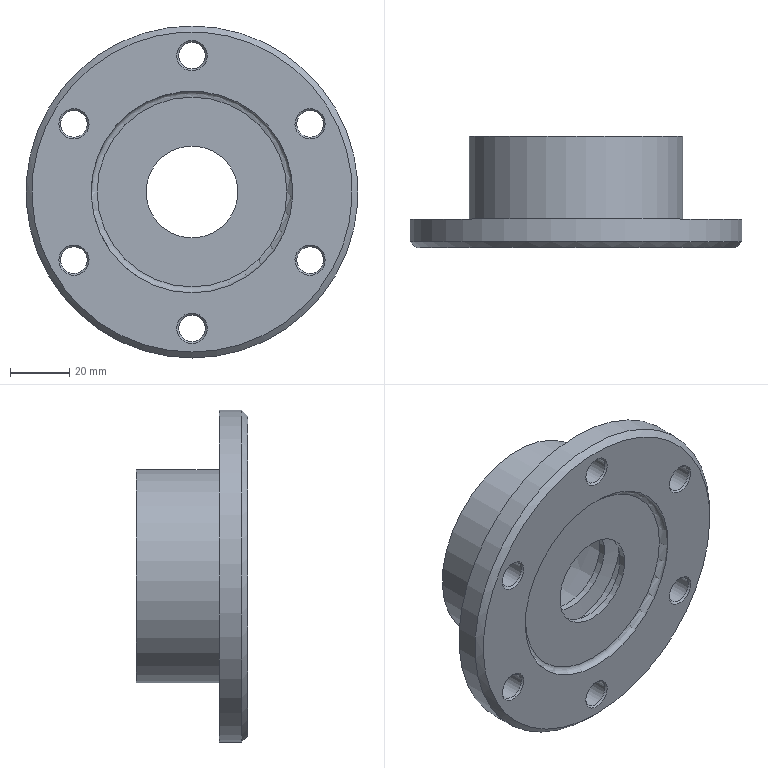Part | NX | 1 solid | 34 faces | box 112 x 37.6 x 112 mm | volume 108254 mm3 | cone 16 | cylinder 11 | plane 5 | torus 2 | commonest cylinder face diameters 9 x6 31 x2 44 x1 72 x1 112 x1
STEP:
#1=CARTESIAN_POINT('',(43.734,-42.624,25.25));
#2=VERTEX_POINT('',#1);
#3=CARTESIAN_POINT('',(39.837,-42.624,23.));
#4=DIRECTION('',(0.,-1.,0.));
#5=DIRECTION('',(0.866,0.,0.5));
#6=AXIS2_PLACEMENT_3D('',#3,#4,#5);
#7=CIRCLE('',#6,4.5);
#8=EDGE_CURVE('',#2,#2,#7,.T.);
#9=ORIENTED_EDGE('',*,*,#8,.F.);
#10=EDGE_LOOP('',(#9));
#11=FACE_BOUND('',#10,.T.);
#12=CARTESIAN_POINT('',(44.254,-43.224,25.55));
#13=VERTEX_POINT('',#12);
#14=CARTESIAN_POINT('',(39.837,-43.224,23.));
#15=DIRECTION('',(0.,1.,0.));
#16=DIRECTION('',(0.866,0.,0.5));
#17=AXIS2_PLACEMENT_3D('',#14,#15,#16);
#18=CIRCLE('',#17,5.1);
#19=EDGE_CURVE('',#13,#13,#18,.T.);
#20=ORIENTED_EDGE('',*,*,#19,.F.);
#21=EDGE_LOOP('',(#20));
#22=FACE_BOUND('',#21,.T.);
#23=CARTESIAN_POINT('',(39.837,-43.224,23.));
#24=DIRECTION('',(0.,-1.,0.));
#25=DIRECTION('',(0.866,0.,0.5));
#26=AXIS2_PLACEMENT_3D('',#23,#24,#25);
#27=CONICAL_SURFACE('',#26,5.1,45.);
#28=ADVANCED_FACE('',(#11,#22),#27,.F.);
#29=CARTESIAN_POINT('',(35.94,-34.224,20.75));
#30=VERTEX_POINT('',#29);
#31=CARTESIAN_POINT('',(39.837,-34.224,23.));
#32=DIRECTION('',(0.,1.,0.));
#33=DIRECTION('',(-0.866,0.,-0.5));
#34=AXIS2_PLACEMENT_3D('',#31,#32,#33);
#35=CIRCLE('',#34,4.5);
#36=EDGE_CURVE('',#30,#30,#35,.T.);
#37=ORIENTED_EDGE('',*,*,#36,.F.);
#38=EDGE_LOOP('',(#37));
#39=FACE_BOUND('',#38,.T.);
#40=CARTESIAN_POINT('',(35.42,-33.624,20.45));
#41=VERTEX_POINT('',#40);
#42=CARTESIAN_POINT('',(39.837,-33.624,23.));
#43=DIRECTION('',(0.,-1.,0.));
#44=DIRECTION('',(-0.866,0.,-0.5));
#45=AXIS2_PLACEMENT_3D('',#42,#43,#44);
#46=CIRCLE('',#45,5.1);
#47=EDGE_CURVE('',#41,#41,#46,.T.);
#48=ORIENTED_EDGE('',*,*,#47,.F.);
#49=EDGE_LOOP('',(#48));
#50=FACE_BOUND('',#49,.T.);
#51=CARTESIAN_POINT('',(39.837,-33.624,23.));
#52=DIRECTION('',(0.,1.,0.));
#53=DIRECTION('',(-0.866,0.,-0.5));
#54=AXIS2_PLACEMENT_3D('',#51,#52,#53);
#55=CONICAL_SURFACE('',#54,5.1,45.);
#56=ADVANCED_FACE('',(#39,#50),#55,.F.);
#57=ORIENTED_EDGE('',*,*,#36,.T.);
#58=EDGE_LOOP('',(#57));
#59=FACE_BOUND('',#58,.T.);
#60=ORIENTED_EDGE('',*,*,#8,.T.);
#61=EDGE_LOOP('',(#60));
#62=FACE_BOUND('',#61,.T.);
#63=CARTESIAN_POINT('',(39.837,-43.224,23.));
#64=DIRECTION('',(0.,1.,0.));
#65=DIRECTION('',(-0.866,0.,-0.5));
#66=AXIS2_PLACEMENT_3D('',#63,#64,#65);
#67=CYLINDRICAL_SURFACE('',#66,4.5);
#68=ADVANCED_FACE('',(#59,#62),#67,.F.);
#69=CARTESIAN_POINT('',(43.734,-42.624,-25.25));
#70=VERTEX_POINT('',#69);
#71=CARTESIAN_POINT('',(39.837,-42.624,-23.));
#72=DIRECTION('',(0.,-1.,0.));
#73=DIRECTION('',(0.866,0.,-0.5));
#74=AXIS2_PLACEMENT_3D('',#71,#72,#73);
#75=CIRCLE('',#74,4.5);
#76=EDGE_CURVE('',#70,#70,#75,.T.);
#77=ORIENTED_EDGE('',*,*,#76,.F.);
#78=EDGE_LOOP('',(#77));
#79=FACE_BOUND('',#78,.T.);
#80=CARTESIAN_POINT('',(44.254,-43.224,-25.55));
#81=VERTEX_POINT('',#80);
#82=CARTESIAN_POINT('',(39.837,-43.224,-23.));
#83=DIRECTION('',(0.,1.,0.));
#84=DIRECTION('',(0.866,0.,-0.5));
#85=AXIS2_PLACEMENT_3D('',#82,#83,#84);
#86=CIRCLE('',#85,5.1);
#87=EDGE_CURVE('',#81,#81,#86,.T.);
#88=ORIENTED_EDGE('',*,*,#87,.F.);
#89=EDGE_LOOP('',(#88));
#90=FACE_BOUND('',#89,.T.);
#91=CARTESIAN_POINT('',(39.837,-43.224,-23.));
#92=DIRECTION('',(0.,-1.,0.));
#93=DIRECTION('',(0.866,0.,-0.5));
#94=AXIS2_PLACEMENT_3D('',#91,#92,#93);
#95=CONICAL_SURFACE('',#94,5.1,45.);
#96=ADVANCED_FACE('',(#79,#90),#95,.F.);
#97=CARTESIAN_POINT('',(35.94,-34.224,-20.75));
#98=VERTEX_POINT('',#97);
#99=CARTESIAN_POINT('',(39.837,-34.224,-23.));
#100=DIRECTION('',(0.,1.,0.));
#101=DIRECTION('',(-0.866,0.,0.5));
#102=AXIS2_PLACEMENT_3D('',#99,#100,#101);
#103=CIRCLE('',#102,4.5);
#104=EDGE_CURVE('',#98,#98,#103,.T.);
#105=ORIENTED_EDGE('',*,*,#104,.F.);
#106=EDGE_LOOP('',(#105));
#107=FACE_BOUND('',#106,.T.);
#108=CARTESIAN_POINT('',(35.42,-33.624,-20.45));
#109=VERTEX_POINT('',#108);
#110=CARTESIAN_POINT('',(39.837,-33.624,-23.));
#111=DIRECTION('',(0.,-1.,0.));
#112=DIRECTION('',(-0.866,0.,0.5));
#113=AXIS2_PLACEMENT_3D('',#110,#111,#112);
#114=CIRCLE('',#113,5.1);
#115=EDGE_CURVE('',#109,#109,#114,.T.);
#116=ORIENTED_EDGE('',*,*,#115,.F.);
#117=EDGE_LOOP('',(#116));
#118=FACE_BOUND('',#117,.T.);
#119=CARTESIAN_POINT('',(39.837,-33.624,-23.));
#120=DIRECTION('',(0.,1.,0.));
#121=DIRECTION('',(-0.866,0.,0.5));
#122=AXIS2_PLACEMENT_3D('',#119,#120,#121);
#123=CONICAL_SURFACE('',#122,5.1,45.);
#124=ADVANCED_FACE('',(#107,#118),#123,.F.);
#125=ORIENTED_EDGE('',*,*,#104,.T.);
#126=EDGE_LOOP('',(#125));
#127=FACE_BOUND('',#126,.T.);
#128=ORIENTED_EDGE('',*,*,#76,.T.);
#129=EDGE_LOOP('',(#128));
#130=FACE_BOUND('',#129,.T.);
#131=CARTESIAN_POINT('',(39.837,-43.224,-23.));
#132=DIRECTION('',(0.,1.,0.));
#133=DIRECTION('',(-0.866,0.,0.5));
#134=AXIS2_PLACEMENT_3D('',#131,#132,#133);
#135=CYLINDRICAL_SURFACE('',#134,4.5);
#136=ADVANCED_FACE('',(#127,#130),#135,.F.);
#137=CARTESIAN_POINT('',(0.,-42.624,-50.5));
#138=VERTEX_POINT('',#137);
#139=CARTESIAN_POINT('',(0.,-42.624,-46.));
#140=DIRECTION('',(0.,-1.,0.));
#141=DIRECTION('',(0.,0.,-1.));
#142=AXIS2_PLACEMENT_3D('',#139,#140,#141);
#143=CIRCLE('',#142,4.5);
#144=EDGE_CURVE('',#138,#138,#143,.T.);
#145=ORIENTED_EDGE('',*,*,#144,.F.);
#146=EDGE_LOOP('',(#145));
#147=FACE_BOUND('',#146,.T.);
#148=CARTESIAN_POINT('',(0.,-43.224,-51.1));
#149=VERTEX_POINT('',#148);
#150=CARTESIAN_POINT('',(0.,-43.224,-46.));
#151=DIRECTION('',(0.,1.,0.));
#152=DIRECTION('',(0.,0.,-1.));
#153=AXIS2_PLACEMENT_3D('',#150,#151,#152);
#154=CIRCLE('',#153,5.1);
#155=EDGE_CURVE('',#149,#149,#154,.T.);
#156=ORIENTED_EDGE('',*,*,#155,.F.);
#157=EDGE_LOOP('',(#156));
#158=FACE_BOUND('',#157,.T.);
#159=CARTESIAN_POINT('',(0.,-43.224,-46.));
#160=DIRECTION('',(0.,-1.,0.));
#161=DIRECTION('',(0.,0.,-1.));
#162=AXIS2_PLACEMENT_3D('',#159,#160,#161);
#163=CONICAL_SURFACE('',#162,5.1,45.);
#164=ADVANCED_FACE('',(#147,#158),#163,.F.);
#165=CARTESIAN_POINT('',(0.,-34.224,-41.5));
#166=VERTEX_POINT('',#165);
#167=CARTESIAN_POINT('',(0.,-34.224,-46.));
#168=DIRECTION('',(0.,1.,0.));
#169=DIRECTION('',(0.,0.,1.));
#170=AXIS2_PLACEMENT_3D('',#167,#168,#169);
#171=CIRCLE('',#170,4.5);
#172=EDGE_CURVE('',#166,#166,#171,.T.);
#173=ORIENTED_EDGE('',*,*,#172,.F.);
#174=EDGE_LOOP('',(#173));
#175=FACE_BOUND('',#174,.T.);
#176=CARTESIAN_POINT('',(0.,-33.624,-40.9));
#177=VERTEX_POINT('',#176);
#178=CARTESIAN_POINT('',(0.,-33.624,-46.));
#179=DIRECTION('',(0.,-1.,0.));
#180=DIRECTION('',(0.,0.,1.));
#181=AXIS2_PLACEMENT_3D('',#178,#179,#180);
#182=CIRCLE('',#181,5.1);
#183=EDGE_CURVE('',#177,#177,#182,.T.);
#184=ORIENTED_EDGE('',*,*,#183,.F.);
#185=EDGE_LOOP('',(#184));
#186=FACE_BOUND('',#185,.T.);
#187=CARTESIAN_POINT('',(0.,-33.624,-46.));
#188=DIRECTION('',(0.,1.,0.));
#189=DIRECTION('',(0.,0.,1.));
#190=AXIS2_PLACEMENT_3D('',#187,#188,#189);
#191=CONICAL_SURFACE('',#190,5.1,45.);
#192=ADVANCED_FACE('',(#175,#186),#191,.F.);
#193=ORIENTED_EDGE('',*,*,#172,.T.);
#194=EDGE_LOOP('',(#193));
#195=FACE_BOUND('',#194,.T.);
#196=ORIENTED_EDGE('',*,*,#144,.T.);
#197=EDGE_LOOP('',(#196));
#198=FACE_BOUND('',#197,.T.);
#199=CARTESIAN_POINT('',(0.,-43.224,-46.));
#200=DIRECTION('',(0.,1.,0.));
#201=DIRECTION('',(0.,0.,1.));
#202=AXIS2_PLACEMENT_3D('',#199,#200,#201);
#203=CYLINDRICAL_SURFACE('',#202,4.5);
#204=ADVANCED_FACE('',(#195,#198),#203,.F.);
#205=CARTESIAN_POINT('',(-43.734,-42.624,-25.25));
#206=VERTEX_POINT('',#205);
#207=CARTESIAN_POINT('',(-39.837,-42.624,-23.));
#208=DIRECTION('',(0.,-1.,0.));
#209=DIRECTION('',(-0.866,0.,-0.5));
#210=AXIS2_PLACEMENT_3D('',#207,#208,#209);
#211=CIRCLE('',#210,4.5);
#212=EDGE_CURVE('',#206,#206,#211,.T.);
#213=ORIENTED_EDGE('',*,*,#212,.F.);
#214=EDGE_LOOP('',(#213));
#215=FACE_BOUND('',#214,.T.);
#216=CARTESIAN_POINT('',(-44.254,-43.224,-25.55));
#217=VERTEX_POINT('',#216);
#218=CARTESIAN_POINT('',(-39.837,-43.224,-23.));
#219=DIRECTION('',(0.,1.,0.));
#220=DIRECTION('',(-0.866,0.,-0.5));
#221=AXIS2_PLACEMENT_3D('',#218,#219,#220);
#222=CIRCLE('',#221,5.1);
#223=EDGE_CURVE('',#217,#217,#222,.T.);
#224=ORIENTED_EDGE('',*,*,#223,.F.);
#225=EDGE_LOOP('',(#224));
#226=FACE_BOUND('',#225,.T.);
#227=CARTESIAN_POINT('',(-39.837,-43.224,-23.));
#228=DIRECTION('',(0.,-1.,0.));
#229=DIRECTION('',(-0.866,0.,-0.5));
#230=AXIS2_PLACEMENT_3D('',#227,#228,#229);
#231=CONICAL_SURFACE('',#230,5.1,45.);
#232=ADVANCED_FACE('',(#215,#226),#231,.F.);
#233=CARTESIAN_POINT('',(-35.94,-34.224,-20.75));
#234=VERTEX_POINT('',#233);
#235=CARTESIAN_POINT('',(-39.837,-34.224,-23.));
#236=DIRECTION('',(0.,1.,0.));
#237=DIRECTION('',(0.866,0.,0.5));
#238=AXIS2_PLACEMENT_3D('',#235,#236,#237);
#239=CIRCLE('',#238,4.5);
#240=EDGE_CURVE('',#234,#234,#239,.T.);
#241=ORIENTED_EDGE('',*,*,#240,.F.);
#242=EDGE_LOOP('',(#241));
#243=FACE_BOUND('',#242,.T.);
#244=CARTESIAN_POINT('',(-35.42,-33.624,-20.45));
#245=VERTEX_POINT('',#244);
#246=CARTESIAN_POINT('',(-39.837,-33.624,-23.));
#247=DIRECTION('',(0.,-1.,0.));
#248=DIRECTION('',(0.866,0.,0.5));
#249=AXIS2_PLACEMENT_3D('',#246,#247,#248);
#250=CIRCLE('',#249,5.1);
#251=EDGE_CURVE('',#245,#245,#250,.T.);
#252=ORIENTED_EDGE('',*,*,#251,.F.);
#253=EDGE_LOOP('',(#252));
#254=FACE_BOUND('',#253,.T.);
#255=CARTESIAN_POINT('',(-39.837,-33.624,-23.));
#256=DIRECTION('',(0.,1.,0.));
#257=DIRECTION('',(0.866,0.,0.5));
#258=AXIS2_PLACEMENT_3D('',#255,#256,#257);
#259=CONICAL_SURFACE('',#258,5.1,45.);
#260=ADVANCED_FACE('',(#243,#254),#259,.F.);
#261=ORIENTED_EDGE('',*,*,#240,.T.);
#262=EDGE_LOOP('',(#261));
#263=FACE_BOUND('',#262,.T.);
#264=ORIENTED_EDGE('',*,*,#212,.T.);
#265=EDGE_LOOP('',(#264));
#266=FACE_BOUND('',#265,.T.);
#267=CARTESIAN_POINT('',(-39.837,-43.224,-23.));
#268=DIRECTION('',(0.,1.,0.));
#269=DIRECTION('',(0.866,0.,0.5));
#270=AXIS2_PLACEMENT_3D('',#267,#268,#269);
#271=CYLINDRICAL_SURFACE('',#270,4.5);
#272=ADVANCED_FACE('',(#263,#266),#271,.F.);
#273=CARTESIAN_POINT('',(-43.734,-42.624,25.25));
#274=VERTEX_POINT('',#273);
#275=CARTESIAN_POINT('',(-39.837,-42.624,23.));
#276=DIRECTION('',(0.,-1.,0.));
#277=DIRECTION('',(-0.866,0.,0.5));
#278=AXIS2_PLACEMENT_3D('',#275,#276,#277);
#279=CIRCLE('',#278,4.5);
#280=EDGE_CURVE('',#274,#274,#279,.T.);
#281=ORIENTED_EDGE('',*,*,#280,.F.);
#282=EDGE_LOOP('',(#281));
#283=FACE_BOUND('',#282,.T.);
#284=CARTESIAN_POINT('',(-44.254,-43.224,25.55));
#285=VERTEX_POINT('',#284);
#286=CARTESIAN_POINT('',(-39.837,-43.224,23.));
#287=DIRECTION('',(0.,1.,0.));
#288=DIRECTION('',(-0.866,0.,0.5));
#289=AXIS2_PLACEMENT_3D('',#286,#287,#288);
#290=CIRCLE('',#289,5.1);
#291=EDGE_CURVE('',#285,#285,#290,.T.);
#292=ORIENTED_EDGE('',*,*,#291,.F.);
#293=EDGE_LOOP('',(#292));
#294=FACE_BOUND('',#293,.T.);
#295=CARTESIAN_POINT('',(-39.837,-43.224,23.));
#296=DIRECTION('',(0.,-1.,0.));
#297=DIRECTION('',(-0.866,0.,0.5));
#298=AXIS2_PLACEMENT_3D('',#295,#296,#297);
#299=CONICAL_SURFACE('',#298,5.1,45.);
#300=ADVANCED_FACE('',(#283,#294),#299,.F.);
#301=CARTESIAN_POINT('',(-35.94,-34.224,20.75));
#302=VERTEX_POINT('',#301);
#303=CARTESIAN_POINT('',(-39.837,-34.224,23.));
#304=DIRECTION('',(0.,1.,0.));
#305=DIRECTION('',(0.866,0.,-0.5));
#306=AXIS2_PLACEMENT_3D('',#303,#304,#305);
#307=CIRCLE('',#306,4.5);
#308=EDGE_CURVE('',#302,#302,#307,.T.);
#309=ORIENTED_EDGE('',*,*,#308,.F.);
#310=EDGE_LOOP('',(#309));
#311=FACE_BOUND('',#310,.T.);
#312=CARTESIAN_POINT('',(-35.42,-33.624,20.45));
#313=VERTEX_POINT('',#312);
#314=CARTESIAN_POINT('',(-39.837,-33.624,23.));
#315=DIRECTION('',(0.,-1.,0.));
#316=DIRECTION('',(0.866,0.,-0.5));
#317=AXIS2_PLACEMENT_3D('',#314,#315,#316);
#318=CIRCLE('',#317,5.1);
#319=EDGE_CURVE('',#313,#313,#318,.T.);
#320=ORIENTED_EDGE('',*,*,#319,.F.);
#321=EDGE_LOOP('',(#320));
#322=FACE_BOUND('',#321,.T.);
#323=CARTESIAN_POINT('',(-39.837,-33.624,23.));
#324=DIRECTION('',(0.,1.,0.));
#325=DIRECTION('',(0.866,0.,-0.5));
#326=AXIS2_PLACEMENT_3D('',#323,#324,#325);
#327=CONICAL_SURFACE('',#326,5.1,45.);
#328=ADVANCED_FACE('',(#311,#322),#327,.F.);
#329=ORIENTED_EDGE('',*,*,#308,.T.);
#330=EDGE_LOOP('',(#329));
#331=FACE_BOUND('',#330,.T.);
#332=ORIENTED_EDGE('',*,*,#280,.T.);
#333=EDGE_LOOP('',(#332));
#334=FACE_BOUND('',#333,.T.);
#335=CARTESIAN_POINT('',(-39.837,-43.224,23.));
#336=DIRECTION('',(0.,1.,0.));
#337=DIRECTION('',(0.866,0.,-0.5));
#338=AXIS2_PLACEMENT_3D('',#335,#336,#337);
#339=CYLINDRICAL_SURFACE('',#338,4.5);
#340=ADVANCED_FACE('',(#331,#334),#339,.F.);
#341=CARTESIAN_POINT('',(0.,-31.426,-15.5));
#342=VERTEX_POINT('',#341);
#343=CARTESIAN_POINT('',(0.,-31.426,0.));
#344=DIRECTION('',(0.,-1.,0.));
#345=DIRECTION('',(0.,0.,-1.));
#346=AXIS2_PLACEMENT_3D('',#343,#344,#345);
#347=CIRCLE('',#346,15.5);
#348=EDGE_CURVE('',#342,#342,#347,.T.);
#349=ORIENTED_EDGE('',*,*,#348,.F.);
#350=EDGE_LOOP('',(#349));
#351=FACE_BOUND('',#350,.T.);
#352=CARTESIAN_POINT('',(0.,-32.224,-22.));
#353=VERTEX_POINT('',#352);
#354=CARTESIAN_POINT('',(0.,-32.224,0.));
#355=DIRECTION('',(0.,-1.,0.));
#356=DIRECTION('',(0.,0.,-1.));
#357=AXIS2_PLACEMENT_3D('',#354,#355,#356);
#358=CIRCLE('',#357,22.);
#359=EDGE_CURVE('',#353,#353,#358,.T.);
#360=ORIENTED_EDGE('',*,*,#359,.T.);
#361=EDGE_LOOP('',(#360));
#362=FACE_BOUND('',#361,.T.);
#363=CARTESIAN_POINT('',(0.,-32.224,0.));
#364=DIRECTION('',(0.,-1.,0.));
#365=DIRECTION('',(0.,0.,1.));
#366=AXIS2_PLACEMENT_3D('',#363,#364,#365);
#367=CONICAL_SURFACE('',#366,22.,83.);
#368=ADVANCED_FACE('',(#351,#362),#367,.F.);
#369=CARTESIAN_POINT('',(0.,-29.224,-15.5));
#370=VERTEX_POINT('',#369);
#371=CARTESIAN_POINT('',(0.,-29.224,0.));
#372=DIRECTION('',(0.,-1.,0.));
#373=DIRECTION('',(0.,0.,-1.));
#374=AXIS2_PLACEMENT_3D('',#371,#372,#373);
#375=CIRCLE('',#374,15.5);
#376=EDGE_CURVE('',#370,#370,#375,.T.);
#377=ORIENTED_EDGE('',*,*,#376,.F.);
#378=EDGE_LOOP('',(#377));
#379=FACE_BOUND('',#378,.T.);
#380=ORIENTED_EDGE('',*,*,#348,.T.);
#381=EDGE_LOOP('',(#380));
#382=FACE_BOUND('',#381,.T.);
#383=CARTESIAN_POINT('',(0.,0.,0.));
#384=DIRECTION('',(0.,-1.,0.));
#385=DIRECTION('',(0.,0.,1.));
#386=AXIS2_PLACEMENT_3D('',#383,#384,#385);
#387=CYLINDRICAL_SURFACE('',#386,15.5);
#388=ADVANCED_FACE('',(#379,#382),#387,.F.);
#389=CARTESIAN_POINT('',(0.,-29.224,-26.564));
#390=VERTEX_POINT('',#389);
#391=CARTESIAN_POINT('',(0.,-29.224,0.));
#392=DIRECTION('',(0.,-1.,0.));
#393=DIRECTION('',(0.,0.,-1.));
#394=AXIS2_PLACEMENT_3D('',#391,#392,#393);
#395=CIRCLE('',#394,26.564);
#396=EDGE_CURVE('',#390,#390,#395,.T.);
#397=ORIENTED_EDGE('',*,*,#396,.F.);
#398=EDGE_LOOP('',(#397));
#399=FACE_BOUND('',#398,.T.);
#400=ORIENTED_EDGE('',*,*,#376,.T.);
#401=EDGE_LOOP('',(#400));
#402=FACE_BOUND('',#401,.T.);
#403=CARTESIAN_POINT('',(-15.5,-29.224,0.));
#404=DIRECTION('',(0.,-1.,0.));
#405=DIRECTION('',(0.,0.,1.));
#406=AXIS2_PLACEMENT_3D('',#403,#404,#405);
#407=PLANE('',#406);
#408=ADVANCED_FACE('',(#399,#402),#407,.F.);
#409=CARTESIAN_POINT('',(0.,-24.474,-31.558));
#410=VERTEX_POINT('',#409);
#411=CARTESIAN_POINT('',(0.,-24.474,0.));
#412=DIRECTION('',(0.,-1.,0.));
#413=DIRECTION('',(0.,0.,-1.));
#414=AXIS2_PLACEMENT_3D('',#411,#412,#413);
#415=CIRCLE('',#414,31.558);
#416=EDGE_CURVE('',#410,#410,#415,.T.);
#417=ORIENTED_EDGE('',*,*,#416,.F.);
#418=EDGE_LOOP('',(#417));
#419=FACE_BOUND('',#418,.T.);
#420=ORIENTED_EDGE('',*,*,#396,.T.);
#421=EDGE_LOOP('',(#420));
#422=FACE_BOUND('',#421,.T.);
#423=CARTESIAN_POINT('',(0.,-24.224,0.));
#424=DIRECTION('',(0.,-1.,0.));
#425=DIRECTION('',(0.,0.,1.));
#426=AXIS2_PLACEMENT_3D('',#423,#424,#425);
#427=TOROIDAL_SURFACE('',#426,26.564,5.);
#428=ADVANCED_FACE('',(#419,#422),#427,.F.);
#429=CARTESIAN_POINT('',(0.,-5.624,-32.5));
#430=VERTEX_POINT('',#429);
#431=CARTESIAN_POINT('',(0.,-5.624,0.));
#432=DIRECTION('',(0.,-1.,0.));
#433=DIRECTION('',(0.,0.,-1.));
#434=AXIS2_PLACEMENT_3D('',#431,#432,#433);
#435=CIRCLE('',#434,32.5);
#436=EDGE_CURVE('',#430,#430,#435,.T.);
#437=ORIENTED_EDGE('',*,*,#436,.F.);
#438=EDGE_LOOP('',(#437));
#439=FACE_BOUND('',#438,.T.);
#440=ORIENTED_EDGE('',*,*,#416,.T.);
#441=EDGE_LOOP('',(#440));
#442=FACE_BOUND('',#441,.T.);
#443=CARTESIAN_POINT('',(0.,-24.474,0.));
#444=DIRECTION('',(0.,1.,0.));
#445=DIRECTION('',(0.,0.,-1.));
#446=AXIS2_PLACEMENT_3D('',#443,#444,#445);
#447=CONICAL_SURFACE('',#446,31.558,2.862);
#448=ADVANCED_FACE('',(#439,#442),#447,.F.);
#449=CARTESIAN_POINT('',(0.,-5.624,-36.));
#450=VERTEX_POINT('',#449);
#451=CARTESIAN_POINT('',(0.,-5.624,0.));
#452=DIRECTION('',(0.,-1.,0.));
#453=DIRECTION('',(0.,0.,-1.));
#454=AXIS2_PLACEMENT_3D('',#451,#452,#453);
#455=CIRCLE('',#454,36.);
#456=EDGE_CURVE('',#450,#450,#455,.T.);
#457=ORIENTED_EDGE('',*,*,#456,.F.);
#458=EDGE_LOOP('',(#457));
#459=FACE_BOUND('',#458,.T.);
#460=ORIENTED_EDGE('',*,*,#436,.T.);
#461=EDGE_LOOP('',(#460));
#462=FACE_BOUND('',#461,.T.);
#463=CARTESIAN_POINT('',(-32.5,-5.624,0.));
#464=DIRECTION('',(0.,-1.,0.));
#465=DIRECTION('',(0.,0.,1.));
#466=AXIS2_PLACEMENT_3D('',#463,#464,#465);
#467=PLANE('',#466);
#468=ADVANCED_FACE('',(#459,#462),#467,.F.);
#469=CARTESIAN_POINT('',(0.,-33.624,-36.));
#470=VERTEX_POINT('',#469);
#471=CARTESIAN_POINT('',(0.,-33.624,0.));
#472=DIRECTION('',(0.,-1.,0.));
#473=DIRECTION('',(0.,0.,-1.));
#474=AXIS2_PLACEMENT_3D('',#471,#472,#473);
#475=CIRCLE('',#474,36.);
#476=EDGE_CURVE('',#470,#470,#475,.T.);
#477=ORIENTED_EDGE('',*,*,#476,.F.);
#478=EDGE_LOOP('',(#477));
#479=FACE_BOUND('',#478,.T.);
#480=ORIENTED_EDGE('',*,*,#456,.T.);
#481=EDGE_LOOP('',(#480));
#482=FACE_BOUND('',#481,.T.);
#483=CARTESIAN_POINT('',(0.,0.,0.));
#484=DIRECTION('',(0.,-1.,0.));
#485=DIRECTION('',(0.,0.,1.));
#486=AXIS2_PLACEMENT_3D('',#483,#484,#485);
#487=CYLINDRICAL_SURFACE('',#486,36.);
#488=ADVANCED_FACE('',(#479,#482),#487,.T.);
#489=ORIENTED_EDGE('',*,*,#47,.T.);
#490=EDGE_LOOP('',(#489));
#491=FACE_BOUND('',#490,.T.);
#492=ORIENTED_EDGE('',*,*,#115,.T.);
#493=EDGE_LOOP('',(#492));
#494=FACE_BOUND('',#493,.T.);
#495=ORIENTED_EDGE('',*,*,#183,.T.);
#496=EDGE_LOOP('',(#495));
#497=FACE_BOUND('',#496,.T.);
#498=ORIENTED_EDGE('',*,*,#251,.T.);
#499=EDGE_LOOP('',(#498));
#500=FACE_BOUND('',#499,.T.);
#501=ORIENTED_EDGE('',*,*,#319,.T.);
#502=EDGE_LOOP('',(#501));
#503=FACE_BOUND('',#502,.T.);
#504=CARTESIAN_POINT('',(0.,-33.624,40.9));
#505=VERTEX_POINT('',#504);
#506=CARTESIAN_POINT('',(0.,-33.624,46.));
#507=DIRECTION('',(0.,-1.,0.));
#508=DIRECTION('',(0.,0.,-1.));
#509=AXIS2_PLACEMENT_3D('',#506,#507,#508);
#510=CIRCLE('',#509,5.1);
#511=EDGE_CURVE('',#505,#505,#510,.T.);
#512=ORIENTED_EDGE('',*,*,#511,.T.);
#513=EDGE_LOOP('',(#512));
#514=FACE_BOUND('',#513,.T.);
#515=CARTESIAN_POINT('',(0.,-33.624,-56.));
#516=VERTEX_POINT('',#515);
#517=CARTESIAN_POINT('',(0.,-33.624,0.));
#518=DIRECTION('',(0.,-1.,0.));
#519=DIRECTION('',(0.,0.,-1.));
#520=AXIS2_PLACEMENT_3D('',#517,#518,#519);
#521=CIRCLE('',#520,56.);
#522=EDGE_CURVE('',#516,#516,#521,.T.);
#523=ORIENTED_EDGE('',*,*,#522,.F.);
#524=EDGE_LOOP('',(#523));
#525=FACE_BOUND('',#524,.T.);
#526=ORIENTED_EDGE('',*,*,#476,.T.);
#527=EDGE_LOOP('',(#526));
#528=FACE_BOUND('',#527,.T.);
#529=CARTESIAN_POINT('',(-36.,-33.624,0.));
#530=DIRECTION('',(0.,-1.,0.));
#531=DIRECTION('',(0.,0.,1.));
#532=AXIS2_PLACEMENT_3D('',#529,#530,#531);
#533=PLANE('',#532);
#534=ADVANCED_FACE('',(#491,#494,#497,#500,#503,#514,#525,#528),#533,.F.);
#535=CARTESIAN_POINT('',(0.,-41.224,-56.));
#536=VERTEX_POINT('',#535);
#537=CARTESIAN_POINT('',(0.,-41.224,0.));
#538=DIRECTION('',(0.,-1.,0.));
#539=DIRECTION('',(0.,0.,-1.));
#540=AXIS2_PLACEMENT_3D('',#537,#538,#539);
#541=CIRCLE('',#540,56.);
#542=EDGE_CURVE('',#536,#536,#541,.T.);
#543=ORIENTED_EDGE('',*,*,#542,.F.);
#544=EDGE_LOOP('',(#543));
#545=FACE_BOUND('',#544,.T.);
#546=ORIENTED_EDGE('',*,*,#522,.T.);
#547=EDGE_LOOP('',(#546));
#548=FACE_BOUND('',#547,.T.);
#549=CARTESIAN_POINT('',(0.,0.,0.));
#550=DIRECTION('',(0.,-1.,0.));
#551=DIRECTION('',(0.,0.,1.));
#552=AXIS2_PLACEMENT_3D('',#549,#550,#551);
#553=CYLINDRICAL_SURFACE('',#552,56.);
#554=ADVANCED_FACE('',(#545,#548),#553,.T.);
#555=CARTESIAN_POINT('',(0.,-43.224,-54.));
#556=VERTEX_POINT('',#555);
#557=CARTESIAN_POINT('',(0.,-43.224,0.));
#558=DIRECTION('',(0.,-1.,0.));
#559=DIRECTION('',(0.,0.,-1.));
#560=AXIS2_PLACEMENT_3D('',#557,#558,#559);
#561=CIRCLE('',#560,54.);
#562=EDGE_CURVE('',#556,#556,#561,.T.);
#563=ORIENTED_EDGE('',*,*,#562,.F.);
#564=EDGE_LOOP('',(#563));
#565=FACE_BOUND('',#564,.T.);
#566=ORIENTED_EDGE('',*,*,#542,.T.);
#567=EDGE_LOOP('',(#566));
#568=FACE_BOUND('',#567,.T.);
#569=CARTESIAN_POINT('',(0.,-41.224,0.));
#570=DIRECTION('',(0.,1.,0.));
#571=DIRECTION('',(0.,0.,-1.));
#572=AXIS2_PLACEMENT_3D('',#569,#570,#571);
#573=CONICAL_SURFACE('',#572,56.,45.);
#574=ADVANCED_FACE('',(#565,#568),#573,.T.);
#575=ORIENTED_EDGE('',*,*,#19,.T.);
#576=EDGE_LOOP('',(#575));
#577=FACE_BOUND('',#576,.T.);
#578=ORIENTED_EDGE('',*,*,#87,.T.);
#579=EDGE_LOOP('',(#578));
#580=FACE_BOUND('',#579,.T.);
#581=ORIENTED_EDGE('',*,*,#155,.T.);
#582=EDGE_LOOP('',(#581));
#583=FACE_BOUND('',#582,.T.);
#584=ORIENTED_EDGE('',*,*,#223,.T.);
#585=EDGE_LOOP('',(#584));
#586=FACE_BOUND('',#585,.T.);
#587=ORIENTED_EDGE('',*,*,#291,.T.);
#588=EDGE_LOOP('',(#587));
#589=FACE_BOUND('',#588,.T.);
#590=CARTESIAN_POINT('',(0.,-43.224,51.1));
#591=VERTEX_POINT('',#590);
#592=CARTESIAN_POINT('',(0.,-43.224,46.));
#593=DIRECTION('',(0.,1.,0.));
#594=DIRECTION('',(0.,0.,1.));
#595=AXIS2_PLACEMENT_3D('',#592,#593,#594);
#596=CIRCLE('',#595,5.1);
#597=EDGE_CURVE('',#591,#591,#596,.T.);
#598=ORIENTED_EDGE('',*,*,#597,.T.);
#599=EDGE_LOOP('',(#598));
#600=FACE_BOUND('',#599,.T.);
#601=CARTESIAN_POINT('',(0.,-43.224,-34.));
#602=VERTEX_POINT('',#601);
#603=CARTESIAN_POINT('',(0.,-43.224,0.));
#604=DIRECTION('',(0.,-1.,0.));
#605=DIRECTION('',(0.,0.,-1.));
#606=AXIS2_PLACEMENT_3D('',#603,#604,#605);
#607=CIRCLE('',#606,34.);
#608=EDGE_CURVE('',#602,#602,#607,.T.);
#609=ORIENTED_EDGE('',*,*,#608,.F.);
#610=EDGE_LOOP('',(#609));
#611=FACE_BOUND('',#610,.T.);
#612=ORIENTED_EDGE('',*,*,#562,.T.);
#613=EDGE_LOOP('',(#612));
#614=FACE_BOUND('',#613,.T.);
#615=CARTESIAN_POINT('',(-47.343,-43.224,0.));
#616=DIRECTION('',(0.,1.,0.));
#617=DIRECTION('',(0.,0.,-1.));
#618=AXIS2_PLACEMENT_3D('',#615,#616,#617);
#619=PLANE('',#618);
#620=ADVANCED_FACE('',(#577,#580,#583,#586,#589,#600,#611,#614),#619,.F.);
#621=CARTESIAN_POINT('',(0.,-41.224,-32.));
#622=VERTEX_POINT('',#621);
#623=CARTESIAN_POINT('',(0.,-41.224,0.));
#624=DIRECTION('',(0.,-1.,0.));
#625=DIRECTION('',(0.,0.,-1.));
#626=AXIS2_PLACEMENT_3D('',#623,#624,#625);
#627=CIRCLE('',#626,32.);
#628=EDGE_CURVE('',#622,#622,#627,.T.);
#629=ORIENTED_EDGE('',*,*,#628,.F.);
#630=EDGE_LOOP('',(#629));
#631=FACE_BOUND('',#630,.T.);
#632=ORIENTED_EDGE('',*,*,#608,.T.);
#633=EDGE_LOOP('',(#632));
#634=FACE_BOUND('',#633,.T.);
#635=CARTESIAN_POINT('',(0.,-43.224,0.));
#636=DIRECTION('',(0.,-1.,0.));
#637=DIRECTION('',(0.,0.,1.));
#638=AXIS2_PLACEMENT_3D('',#635,#636,#637);
#639=TOROIDAL_SURFACE('',#638,32.,2.);
#640=ADVANCED_FACE('',(#631,#634),#639,.F.);
#641=CARTESIAN_POINT('',(0.,-41.224,-15.5));
#642=VERTEX_POINT('',#641);
#643=CARTESIAN_POINT('',(0.,-41.224,0.));
#644=DIRECTION('',(0.,-1.,0.));
#645=DIRECTION('',(0.,0.,-1.));
#646=AXIS2_PLACEMENT_3D('',#643,#644,#645);
#647=CIRCLE('',#646,15.5);
#648=EDGE_CURVE('',#642,#642,#647,.T.);
#649=ORIENTED_EDGE('',*,*,#648,.F.);
#650=EDGE_LOOP('',(#649));
#651=FACE_BOUND('',#650,.T.);
#652=ORIENTED_EDGE('',*,*,#628,.T.);
#653=EDGE_LOOP('',(#652));
#654=FACE_BOUND('',#653,.T.);
#655=CARTESIAN_POINT('',(-32.,-41.224,0.));
#656=DIRECTION('',(0.,1.,0.));
#657=DIRECTION('',(0.,0.,-1.));
#658=AXIS2_PLACEMENT_3D('',#655,#656,#657);
#659=PLANE('',#658);
#660=ADVANCED_FACE('',(#651,#654),#659,.F.);
#661=CARTESIAN_POINT('',(0.,-39.022,-15.5));
#662=VERTEX_POINT('',#661);
#663=CARTESIAN_POINT('',(0.,-39.022,0.));
#664=DIRECTION('',(0.,-1.,0.));
#665=DIRECTION('',(0.,0.,-1.));
#666=AXIS2_PLACEMENT_3D('',#663,#664,#665);
#667=CIRCLE('',#666,15.5);
#668=EDGE_CURVE('',#662,#662,#667,.T.);
#669=ORIENTED_EDGE('',*,*,#668,.F.);
#670=EDGE_LOOP('',(#669));
#671=FACE_BOUND('',#670,.T.);
#672=ORIENTED_EDGE('',*,*,#648,.T.);
#673=EDGE_LOOP('',(#672));
#674=FACE_BOUND('',#673,.T.);
#675=CARTESIAN_POINT('',(0.,0.,0.));
#676=DIRECTION('',(0.,-1.,0.));
#677=DIRECTION('',(0.,0.,1.));
#678=AXIS2_PLACEMENT_3D('',#675,#676,#677);
#679=CYLINDRICAL_SURFACE('',#678,15.5);
#680=ADVANCED_FACE('',(#671,#674),#679,.F.);
#681=CARTESIAN_POINT('',(0.,-38.224,-22.));
#682=VERTEX_POINT('',#681);
#683=CARTESIAN_POINT('',(0.,-38.224,0.));
#684=DIRECTION('',(0.,-1.,0.));
#685=DIRECTION('',(0.,0.,-1.));
#686=AXIS2_PLACEMENT_3D('',#683,#684,#685);
#687=CIRCLE('',#686,22.);
#688=EDGE_CURVE('',#682,#682,#687,.T.);
#689=ORIENTED_EDGE('',*,*,#688,.F.);
#690=EDGE_LOOP('',(#689));
#691=FACE_BOUND('',#690,.T.);
#692=ORIENTED_EDGE('',*,*,#668,.T.);
#693=EDGE_LOOP('',(#692));
#694=FACE_BOUND('',#693,.T.);
#695=CARTESIAN_POINT('',(0.,-39.022,0.));
#696=DIRECTION('',(0.,1.,0.));
#697=DIRECTION('',(0.,0.,-1.));
#698=AXIS2_PLACEMENT_3D('',#695,#696,#697);
#699=CONICAL_SURFACE('',#698,15.5,83.);
#700=ADVANCED_FACE('',(#691,#694),#699,.F.);
#701=ORIENTED_EDGE('',*,*,#359,.F.);
#702=EDGE_LOOP('',(#701));
#703=FACE_BOUND('',#702,.T.);
#704=ORIENTED_EDGE('',*,*,#688,.T.);
#705=EDGE_LOOP('',(#704));
#706=FACE_BOUND('',#705,.T.);
#707=CARTESIAN_POINT('',(0.,0.,0.));
#708=DIRECTION('',(0.,-1.,0.));
#709=DIRECTION('',(0.,0.,1.));
#710=AXIS2_PLACEMENT_3D('',#707,#708,#709);
#711=CYLINDRICAL_SURFACE('',#710,22.);
#712=ADVANCED_FACE('',(#703,#706),#711,.F.);
#713=CARTESIAN_POINT('',(0.,-34.224,41.5));
#714=VERTEX_POINT('',#713);
#715=CARTESIAN_POINT('',(0.,-34.224,46.));
#716=DIRECTION('',(0.,1.,0.));
#717=DIRECTION('',(0.,0.,-1.));
#718=AXIS2_PLACEMENT_3D('',#715,#716,#717);
#719=CIRCLE('',#718,4.5);
#720=EDGE_CURVE('',#714,#714,#719,.T.);
#721=ORIENTED_EDGE('',*,*,#720,.T.);
#722=EDGE_LOOP('',(#721));
#723=FACE_BOUND('',#722,.T.);
#724=CARTESIAN_POINT('',(0.,-42.624,50.5));
#725=VERTEX_POINT('',#724);
#726=CARTESIAN_POINT('',(0.,-42.624,46.));
#727=DIRECTION('',(0.,-1.,0.));
#728=DIRECTION('',(0.,0.,1.));
#729=AXIS2_PLACEMENT_3D('',#726,#727,#728);
#730=CIRCLE('',#729,4.5);
#731=EDGE_CURVE('',#725,#725,#730,.T.);
#732=ORIENTED_EDGE('',*,*,#731,.T.);
#733=EDGE_LOOP('',(#732));
#734=FACE_BOUND('',#733,.T.);
#735=CARTESIAN_POINT('',(0.,-43.224,46.));
#736=DIRECTION('',(0.,1.,0.));
#737=DIRECTION('',(0.,0.,-1.));
#738=AXIS2_PLACEMENT_3D('',#735,#736,#737);
#739=CYLINDRICAL_SURFACE('',#738,4.5);
#740=ADVANCED_FACE('',(#723,#734),#739,.F.);
#741=ORIENTED_EDGE('',*,*,#731,.F.);
#742=EDGE_LOOP('',(#741));
#743=FACE_BOUND('',#742,.T.);
#744=ORIENTED_EDGE('',*,*,#597,.F.);
#745=EDGE_LOOP('',(#744));
#746=FACE_BOUND('',#745,.T.);
#747=CARTESIAN_POINT('',(0.,-43.224,46.));
#748=DIRECTION('',(0.,-1.,0.));
#749=DIRECTION('',(0.,0.,1.));
#750=AXIS2_PLACEMENT_3D('',#747,#748,#749);
#751=CONICAL_SURFACE('',#750,5.1,45.);
#752=ADVANCED_FACE('',(#743,#746),#751,.F.);
#753=ORIENTED_EDGE('',*,*,#720,.F.);
#754=EDGE_LOOP('',(#753));
#755=FACE_BOUND('',#754,.T.);
#756=ORIENTED_EDGE('',*,*,#511,.F.);
#757=EDGE_LOOP('',(#756));
#758=FACE_BOUND('',#757,.T.);
#759=CARTESIAN_POINT('',(0.,-33.624,46.));
#760=DIRECTION('',(0.,1.,0.));
#761=DIRECTION('',(0.,0.,-1.));
#762=AXIS2_PLACEMENT_3D('',#759,#760,#761);
#763=CONICAL_SURFACE('',#762,5.1,45.);
#764=ADVANCED_FACE('',(#755,#758),#763,.F.);
#765=CLOSED_SHELL('',(#28,#56,#68,#96,#124,#136,#164,#192,#204,#232,#260,#272,#300,#328,#340,#368,#388,#408,#428,#448,#468,#488,#534,#554,#574,#620,#640,#660,#680,#700,#712,#740,#752,#764));
#766=MANIFOLD_SOLID_BREP('',#765);
#767=(LENGTH_UNIT()NAMED_UNIT(*)SI_UNIT(.MILLI.,.METRE.));
#768=UNCERTAINTY_MEASURE_WITH_UNIT(LENGTH_MEASURE(0.00002),#767,'','');
#769=(NAMED_UNIT(*)PLANE_ANGLE_UNIT()SI_UNIT($,.RADIAN.));
#770=PLANE_ANGLE_MEASURE_WITH_UNIT(PLANE_ANGLE_MEASURE(0.01745),#769);
#771=DIMENSIONAL_EXPONENTS(0.,0.,0.,0.,0.,0.,0.);
#772=(CONVERSION_BASED_UNIT('DEGREE',#770)NAMED_UNIT(#771)PLANE_ANGLE_UNIT());
#773=(NAMED_UNIT(*)SI_UNIT($,.STERADIAN.)SOLID_ANGLE_UNIT());
#774=(GEOMETRIC_REPRESENTATION_CONTEXT(3)GLOBAL_UNCERTAINTY_ASSIGNED_CONTEXT((#768))GLOBAL_UNIT_ASSIGNED_CONTEXT((#767,#772,#773))REPRESENTATION_CONTEXT('',''));
#775=ADVANCED_BREP_SHAPE_REPRESENTATION('',(#766),#774);